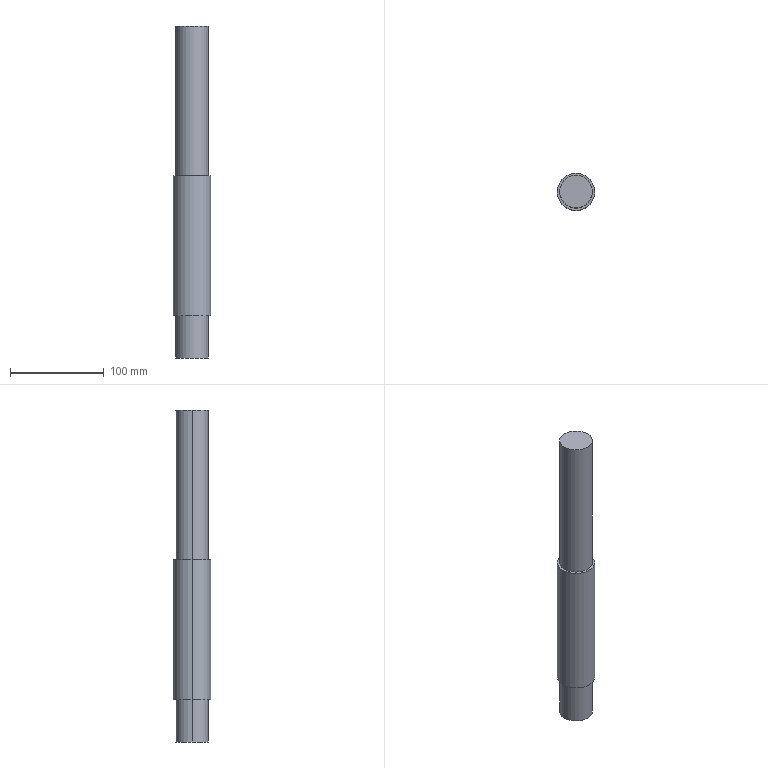Part | SolidWorks | features ICE 2, Extrusion 1 | 1 solid | 10 faces | box 40 x 40 x 355 mm | volume 385729 mm3 | cylinder 6 | plane 4 | commonest cylinder face diameters 35 x4 40 x2
STEP:
#1=CARTESIAN_POINT('',(-17.5,0.,-45.));
#2=VERTEX_POINT('',#1);
#3=CARTESIAN_POINT('',(17.5,0.,-45.));
#4=VERTEX_POINT('',#3);
#5=CARTESIAN_POINT('',(0.,0.,-45.));
#6=DIRECTION('',(0.,0.,-1.));
#7=DIRECTION('',(-1.,0.,0.));
#8=AXIS2_PLACEMENT_3D('',#5,#6,#7);
#9=CIRCLE('',#8,17.5);
#10=EDGE_CURVE('',#2,#4,#9,.T.);
#11=ORIENTED_EDGE('',*,*,#10,.F.);
#12=CARTESIAN_POINT('',(-17.5,0.,0.));
#13=VERTEX_POINT('',#12);
#14=CARTESIAN_POINT('',(-17.5,0.,-45.));
#15=DIRECTION('',(0.,0.,1.));
#16=VECTOR('',#15,1000.);
#17=LINE('',#14,#16);
#18=EDGE_CURVE('',#2,#13,#17,.T.);
#19=ORIENTED_EDGE('',*,*,#18,.T.);
#20=CARTESIAN_POINT('',(17.5,0.,0.));
#21=VERTEX_POINT('',#20);
#22=CARTESIAN_POINT('',(0.,0.,0.));
#23=DIRECTION('',(0.,0.,-1.));
#24=DIRECTION('',(-1.,0.,0.));
#25=AXIS2_PLACEMENT_3D('',#22,#23,#24);
#26=CIRCLE('',#25,17.5);
#27=EDGE_CURVE('',#13,#21,#26,.T.);
#28=ORIENTED_EDGE('',*,*,#27,.T.);
#29=CARTESIAN_POINT('',(17.5,0.,-45.));
#30=DIRECTION('',(0.,0.,1.));
#31=VECTOR('',#30,1000.);
#32=LINE('',#29,#31);
#33=EDGE_CURVE('',#4,#21,#32,.T.);
#34=ORIENTED_EDGE('',*,*,#33,.F.);
#35=EDGE_LOOP('',(#11,#19,#28,#34));
#36=FACE_OUTER_BOUND('',#35,.T.);
#37=CARTESIAN_POINT('',(0.,0.,-45.));
#38=DIRECTION('',(0.,0.,1.));
#39=DIRECTION('',(1.,0.,0.));
#40=AXIS2_PLACEMENT_3D('',#37,#38,#39);
#41=CYLINDRICAL_SURFACE('',#40,17.5);
#42=ADVANCED_FACE('',(#36),#41,.T.);
#43=CARTESIAN_POINT('',(17.5,0.,310.));
#44=VERTEX_POINT('',#43);
#45=CARTESIAN_POINT('',(-17.5,0.,310.));
#46=VERTEX_POINT('',#45);
#47=CARTESIAN_POINT('',(0.,0.,310.));
#48=DIRECTION('',(0.,0.,1.));
#49=DIRECTION('',(1.,0.,0.));
#50=AXIS2_PLACEMENT_3D('',#47,#48,#49);
#51=CIRCLE('',#50,17.5);
#52=EDGE_CURVE('',#44,#46,#51,.T.);
#53=ORIENTED_EDGE('',*,*,#52,.F.);
#54=CARTESIAN_POINT('',(17.5,0.,150.));
#55=VERTEX_POINT('',#54);
#56=CARTESIAN_POINT('',(17.5,0.,310.));
#57=DIRECTION('',(0.,0.,-1.));
#58=VECTOR('',#57,1000.);
#59=LINE('',#56,#58);
#60=EDGE_CURVE('',#44,#55,#59,.T.);
#61=ORIENTED_EDGE('',*,*,#60,.T.);
#62=CARTESIAN_POINT('',(-17.5,0.,150.));
#63=VERTEX_POINT('',#62);
#64=CARTESIAN_POINT('',(0.,0.,150.));
#65=DIRECTION('',(0.,0.,1.));
#66=DIRECTION('',(1.,0.,0.));
#67=AXIS2_PLACEMENT_3D('',#64,#65,#66);
#68=CIRCLE('',#67,17.5);
#69=EDGE_CURVE('',#55,#63,#68,.T.);
#70=ORIENTED_EDGE('',*,*,#69,.T.);
#71=CARTESIAN_POINT('',(-17.5,0.,310.));
#72=DIRECTION('',(0.,0.,-1.));
#73=VECTOR('',#72,1000.);
#74=LINE('',#71,#73);
#75=EDGE_CURVE('',#46,#63,#74,.T.);
#76=ORIENTED_EDGE('',*,*,#75,.F.);
#77=EDGE_LOOP('',(#53,#61,#70,#76));
#78=FACE_OUTER_BOUND('',#77,.T.);
#79=CARTESIAN_POINT('',(0.,0.,310.));
#80=DIRECTION('',(0.,0.,-1.));
#81=DIRECTION('',(-1.,0.,0.));
#82=AXIS2_PLACEMENT_3D('',#79,#80,#81);
#83=CYLINDRICAL_SURFACE('',#82,17.5);
#84=ADVANCED_FACE('',(#78),#83,.T.);
#85=CARTESIAN_POINT('',(20.,0.,150.));
#86=VERTEX_POINT('',#85);
#87=CARTESIAN_POINT('',(-20.,0.,150.));
#88=VERTEX_POINT('',#87);
#89=CARTESIAN_POINT('',(0.,0.,150.));
#90=DIRECTION('',(0.,0.,1.));
#91=DIRECTION('',(1.,0.,0.));
#92=AXIS2_PLACEMENT_3D('',#89,#90,#91);
#93=CIRCLE('',#92,20.);
#94=EDGE_CURVE('',#86,#88,#93,.T.);
#95=ORIENTED_EDGE('',*,*,#94,.F.);
#96=CARTESIAN_POINT('',(20.,0.,0.));
#97=VERTEX_POINT('',#96);
#98=CARTESIAN_POINT('',(20.,0.,150.));
#99=DIRECTION('',(0.,0.,-1.));
#100=VECTOR('',#99,1000.);
#101=LINE('',#98,#100);
#102=EDGE_CURVE('',#86,#97,#101,.T.);
#103=ORIENTED_EDGE('',*,*,#102,.T.);
#104=CARTESIAN_POINT('',(-20.,0.,0.));
#105=VERTEX_POINT('',#104);
#106=CARTESIAN_POINT('',(0.,0.,0.));
#107=DIRECTION('',(0.,0.,1.));
#108=DIRECTION('',(1.,0.,0.));
#109=AXIS2_PLACEMENT_3D('',#106,#107,#108);
#110=CIRCLE('',#109,20.);
#111=EDGE_CURVE('',#97,#105,#110,.T.);
#112=ORIENTED_EDGE('',*,*,#111,.T.);
#113=CARTESIAN_POINT('',(-20.,0.,150.));
#114=DIRECTION('',(0.,0.,-1.));
#115=VECTOR('',#114,1000.);
#116=LINE('',#113,#115);
#117=EDGE_CURVE('',#88,#105,#116,.T.);
#118=ORIENTED_EDGE('',*,*,#117,.F.);
#119=EDGE_LOOP('',(#95,#103,#112,#118));
#120=FACE_OUTER_BOUND('',#119,.T.);
#121=CARTESIAN_POINT('',(0.,0.,150.));
#122=DIRECTION('',(0.,0.,-1.));
#123=DIRECTION('',(-1.,0.,0.));
#124=AXIS2_PLACEMENT_3D('',#121,#122,#123);
#125=CYLINDRICAL_SURFACE('',#124,20.);
#126=ADVANCED_FACE('',(#120),#125,.T.);
#127=ORIENTED_EDGE('',*,*,#102,.F.);
#128=CARTESIAN_POINT('',(0.,0.,150.));
#129=DIRECTION('',(0.,0.,1.));
#130=DIRECTION('',(1.,0.,0.));
#131=AXIS2_PLACEMENT_3D('',#128,#129,#130);
#132=CIRCLE('',#131,20.);
#133=EDGE_CURVE('',#88,#86,#132,.T.);
#134=ORIENTED_EDGE('',*,*,#133,.F.);
#135=ORIENTED_EDGE('',*,*,#117,.T.);
#136=CARTESIAN_POINT('',(0.,0.,0.));
#137=DIRECTION('',(0.,0.,1.));
#138=DIRECTION('',(1.,0.,0.));
#139=AXIS2_PLACEMENT_3D('',#136,#137,#138);
#140=CIRCLE('',#139,20.);
#141=EDGE_CURVE('',#105,#97,#140,.T.);
#142=ORIENTED_EDGE('',*,*,#141,.T.);
#143=EDGE_LOOP('',(#127,#134,#135,#142));
#144=FACE_OUTER_BOUND('',#143,.T.);
#145=CARTESIAN_POINT('',(0.,0.,150.));
#146=DIRECTION('',(0.,0.,-1.));
#147=DIRECTION('',(-1.,0.,0.));
#148=AXIS2_PLACEMENT_3D('',#145,#146,#147);
#149=CYLINDRICAL_SURFACE('',#148,20.);
#150=ADVANCED_FACE('',(#144),#149,.T.);
#151=CARTESIAN_POINT('',(0.,0.,150.));
#152=DIRECTION('',(0.,0.,1.));
#153=DIRECTION('',(1.,0.,0.));
#154=AXIS2_PLACEMENT_3D('',#151,#152,#153);
#155=CIRCLE('',#154,17.5);
#156=EDGE_CURVE('',#63,#55,#155,.T.);
#157=ORIENTED_EDGE('',*,*,#156,.F.);
#158=ORIENTED_EDGE('',*,*,#69,.F.);
#159=EDGE_LOOP('',(#157,#158));
#160=FACE_BOUND('',#159,.T.);
#161=ORIENTED_EDGE('',*,*,#133,.T.);
#162=ORIENTED_EDGE('',*,*,#94,.T.);
#163=EDGE_LOOP('',(#161,#162));
#164=FACE_OUTER_BOUND('',#163,.T.);
#165=CARTESIAN_POINT('',(0.,0.,150.));
#166=DIRECTION('',(0.,0.,1.));
#167=DIRECTION('',(1.,0.,0.));
#168=AXIS2_PLACEMENT_3D('',#165,#166,#167);
#169=PLANE('',#168);
#170=ADVANCED_FACE('',(#160,#164),#169,.T.);
#171=CARTESIAN_POINT('',(0.,0.,0.));
#172=DIRECTION('',(0.,0.,-1.));
#173=DIRECTION('',(-1.,0.,0.));
#174=AXIS2_PLACEMENT_3D('',#171,#172,#173);
#175=CIRCLE('',#174,17.5);
#176=EDGE_CURVE('',#21,#13,#175,.T.);
#177=ORIENTED_EDGE('',*,*,#176,.F.);
#178=ORIENTED_EDGE('',*,*,#27,.F.);
#179=EDGE_LOOP('',(#177,#178));
#180=FACE_BOUND('',#179,.T.);
#181=ORIENTED_EDGE('',*,*,#141,.F.);
#182=ORIENTED_EDGE('',*,*,#111,.F.);
#183=EDGE_LOOP('',(#181,#182));
#184=FACE_OUTER_BOUND('',#183,.T.);
#185=CARTESIAN_POINT('',(0.,0.,0.));
#186=DIRECTION('',(0.,0.,1.));
#187=DIRECTION('',(1.,0.,0.));
#188=AXIS2_PLACEMENT_3D('',#185,#186,#187);
#189=PLANE('',#188);
#190=ADVANCED_FACE('',(#180,#184),#189,.F.);
#191=ORIENTED_EDGE('',*,*,#60,.F.);
#192=CARTESIAN_POINT('',(0.,0.,310.));
#193=DIRECTION('',(0.,0.,1.));
#194=DIRECTION('',(1.,0.,0.));
#195=AXIS2_PLACEMENT_3D('',#192,#193,#194);
#196=CIRCLE('',#195,17.5);
#197=EDGE_CURVE('',#46,#44,#196,.T.);
#198=ORIENTED_EDGE('',*,*,#197,.F.);
#199=ORIENTED_EDGE('',*,*,#75,.T.);
#200=ORIENTED_EDGE('',*,*,#156,.T.);
#201=EDGE_LOOP('',(#191,#198,#199,#200));
#202=FACE_OUTER_BOUND('',#201,.T.);
#203=CARTESIAN_POINT('',(0.,0.,310.));
#204=DIRECTION('',(0.,0.,-1.));
#205=DIRECTION('',(-1.,0.,0.));
#206=AXIS2_PLACEMENT_3D('',#203,#204,#205);
#207=CYLINDRICAL_SURFACE('',#206,17.5);
#208=ADVANCED_FACE('',(#202),#207,.T.);
#209=ORIENTED_EDGE('',*,*,#197,.T.);
#210=ORIENTED_EDGE('',*,*,#52,.T.);
#211=EDGE_LOOP('',(#209,#210));
#212=FACE_OUTER_BOUND('',#211,.T.);
#213=CARTESIAN_POINT('',(0.,0.,310.));
#214=DIRECTION('',(0.,0.,1.));
#215=DIRECTION('',(1.,0.,0.));
#216=AXIS2_PLACEMENT_3D('',#213,#214,#215);
#217=PLANE('',#216);
#218=ADVANCED_FACE('',(#212),#217,.T.);
#219=ORIENTED_EDGE('',*,*,#18,.F.);
#220=CARTESIAN_POINT('',(0.,0.,-45.));
#221=DIRECTION('',(0.,0.,-1.));
#222=DIRECTION('',(-1.,0.,0.));
#223=AXIS2_PLACEMENT_3D('',#220,#221,#222);
#224=CIRCLE('',#223,17.5);
#225=EDGE_CURVE('',#4,#2,#224,.T.);
#226=ORIENTED_EDGE('',*,*,#225,.F.);
#227=ORIENTED_EDGE('',*,*,#33,.T.);
#228=ORIENTED_EDGE('',*,*,#176,.T.);
#229=EDGE_LOOP('',(#219,#226,#227,#228));
#230=FACE_OUTER_BOUND('',#229,.T.);
#231=CARTESIAN_POINT('',(0.,0.,-45.));
#232=DIRECTION('',(0.,0.,1.));
#233=DIRECTION('',(1.,0.,0.));
#234=AXIS2_PLACEMENT_3D('',#231,#232,#233);
#235=CYLINDRICAL_SURFACE('',#234,17.5);
#236=ADVANCED_FACE('',(#230),#235,.T.);
#237=ORIENTED_EDGE('',*,*,#225,.T.);
#238=ORIENTED_EDGE('',*,*,#10,.T.);
#239=EDGE_LOOP('',(#237,#238));
#240=FACE_OUTER_BOUND('',#239,.T.);
#241=CARTESIAN_POINT('',(0.,0.,-45.));
#242=DIRECTION('',(0.,0.,-1.));
#243=DIRECTION('',(-1.,0.,0.));
#244=AXIS2_PLACEMENT_3D('',#241,#242,#243);
#245=PLANE('',#244);
#246=ADVANCED_FACE('',(#240),#245,.T.);
#247=CLOSED_SHELL('',(#42,#84,#126,#150,#170,#190,#208,#218,#236,#246));
#248=MANIFOLD_SOLID_BREP('',#247);
#249=CARTESIAN_POINT('',(0.,0.,0.));
#250=DIRECTION('',(0.,0.,1.));
#251=DIRECTION('',(1.,0.,0.));
#252=AXIS2_PLACEMENT_3D('',#249,#250,#251);
#253=(LENGTH_UNIT()NAMED_UNIT(*)SI_UNIT(.MILLI.,.METRE.));
#254=UNCERTAINTY_MEASURE_WITH_UNIT(LENGTH_MEASURE(0.00001),#253,'','');
#255=(NAMED_UNIT(*)PLANE_ANGLE_UNIT()SI_UNIT($,.RADIAN.));
#256=(NAMED_UNIT(*)SI_UNIT($,.STERADIAN.)SOLID_ANGLE_UNIT());
#257=(GEOMETRIC_REPRESENTATION_CONTEXT(3)GLOBAL_UNCERTAINTY_ASSIGNED_CONTEXT((#254))GLOBAL_UNIT_ASSIGNED_CONTEXT((#253,#255,#256))REPRESENTATION_CONTEXT('',''));
#258=ADVANCED_BREP_SHAPE_REPRESENTATION('',(#248,#252),#257);